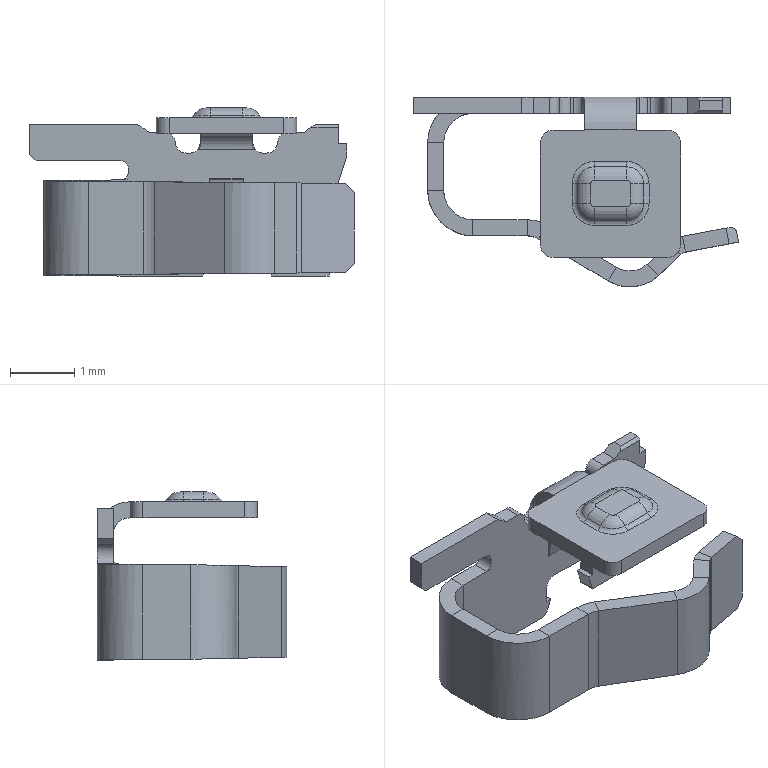Part | NX | 1 solid | 143 faces | box 5.066 x 2.959 x 2.622 mm | volume 5.796 mm3 | plane 91 | cylinder 38 | torus 12 | spline 2 | commonest cylinder face diameters 0.3 x6 0.2 x5 0.5 x5 0.7 x5 0.35 x4 0.4 x4